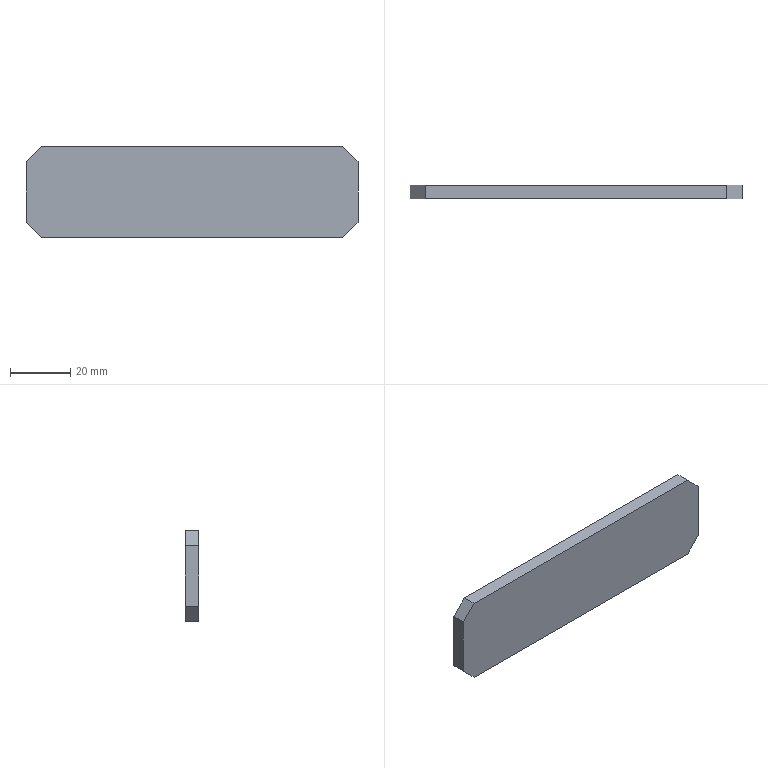Part | SolidWorks | features FlatPattern 1, SMBaseFlange 1, SheetMetal 1 | 1 solid | 10 faces | box 110 x 4.5 x 30 mm | volume 14625 mm3 | plane 10
STEP:
#1=CARTESIAN_POINT('',(-55.,0.,-10.));
#2=VERTEX_POINT('',#1);
#3=CARTESIAN_POINT('',(-55.,0.,10.));
#4=VERTEX_POINT('',#3);
#5=CARTESIAN_POINT('',(-55.,0.,-10.));
#6=DIRECTION('',(0.,0.,1.));
#7=VECTOR('',#6,1000.);
#8=LINE('',#5,#7);
#9=EDGE_CURVE('',#2,#4,#8,.T.);
#10=ORIENTED_EDGE('',*,*,#9,.F.);
#11=CARTESIAN_POINT('',(-55.,-4.5,-10.));
#12=VERTEX_POINT('',#11);
#13=CARTESIAN_POINT('',(-55.,-4.5,-10.));
#14=DIRECTION('',(0.,1.,0.));
#15=VECTOR('',#14,1000.);
#16=LINE('',#13,#15);
#17=EDGE_CURVE('',#12,#2,#16,.T.);
#18=ORIENTED_EDGE('',*,*,#17,.F.);
#19=CARTESIAN_POINT('',(-55.,-4.5,10.));
#20=VERTEX_POINT('',#19);
#21=CARTESIAN_POINT('',(-55.,-4.5,-10.));
#22=DIRECTION('',(0.,0.,1.));
#23=VECTOR('',#22,1000.);
#24=LINE('',#21,#23);
#25=EDGE_CURVE('',#12,#20,#24,.T.);
#26=ORIENTED_EDGE('',*,*,#25,.T.);
#27=CARTESIAN_POINT('',(-55.,-4.5,10.));
#28=DIRECTION('',(0.,1.,0.));
#29=VECTOR('',#28,1000.);
#30=LINE('',#27,#29);
#31=EDGE_CURVE('',#20,#4,#30,.T.);
#32=ORIENTED_EDGE('',*,*,#31,.T.);
#33=EDGE_LOOP('',(#10,#18,#26,#32));
#34=FACE_OUTER_BOUND('',#33,.T.);
#35=CARTESIAN_POINT('',(-55.,-4.5,-10.));
#36=DIRECTION('',(-1.,0.,0.));
#37=DIRECTION('',(0.,0.,1.));
#38=AXIS2_PLACEMENT_3D('',#35,#36,#37);
#39=PLANE('',#38);
#40=ADVANCED_FACE('',(#34),#39,.T.);
#41=CARTESIAN_POINT('',(-50.,0.,-15.));
#42=VERTEX_POINT('',#41);
#43=CARTESIAN_POINT('',(-55.,0.,-10.));
#44=DIRECTION('',(-0.7071,0.,0.7071));
#45=VECTOR('',#44,1000.);
#46=LINE('',#43,#45);
#47=EDGE_CURVE('',#42,#2,#46,.T.);
#48=ORIENTED_EDGE('',*,*,#47,.F.);
#49=CARTESIAN_POINT('',(-50.,-4.5,-15.));
#50=VERTEX_POINT('',#49);
#51=CARTESIAN_POINT('',(-50.,-4.5,-15.));
#52=DIRECTION('',(0.,1.,0.));
#53=VECTOR('',#52,1000.);
#54=LINE('',#51,#53);
#55=EDGE_CURVE('',#50,#42,#54,.T.);
#56=ORIENTED_EDGE('',*,*,#55,.F.);
#57=CARTESIAN_POINT('',(-55.,-4.5,-10.));
#58=DIRECTION('',(-0.7071,0.,0.7071));
#59=VECTOR('',#58,1000.);
#60=LINE('',#57,#59);
#61=EDGE_CURVE('',#50,#12,#60,.T.);
#62=ORIENTED_EDGE('',*,*,#61,.T.);
#63=ORIENTED_EDGE('',*,*,#17,.T.);
#64=EDGE_LOOP('',(#48,#56,#62,#63));
#65=FACE_OUTER_BOUND('',#64,.T.);
#66=CARTESIAN_POINT('',(-55.,-4.5,-10.));
#67=DIRECTION('',(-0.7071,0.,-0.7071));
#68=DIRECTION('',(-0.7071,0.,0.7071));
#69=AXIS2_PLACEMENT_3D('',#66,#67,#68);
#70=PLANE('',#69);
#71=ADVANCED_FACE('',(#65),#70,.T.);
#72=CARTESIAN_POINT('',(50.,0.,-15.));
#73=VERTEX_POINT('',#72);
#74=CARTESIAN_POINT('',(-50.,0.,-15.));
#75=DIRECTION('',(-1.,0.,0.));
#76=VECTOR('',#75,1000.);
#77=LINE('',#74,#76);
#78=EDGE_CURVE('',#73,#42,#77,.T.);
#79=ORIENTED_EDGE('',*,*,#78,.F.);
#80=CARTESIAN_POINT('',(50.,-4.5,-15.));
#81=VERTEX_POINT('',#80);
#82=CARTESIAN_POINT('',(50.,-4.5,-15.));
#83=DIRECTION('',(0.,1.,0.));
#84=VECTOR('',#83,1000.);
#85=LINE('',#82,#84);
#86=EDGE_CURVE('',#81,#73,#85,.T.);
#87=ORIENTED_EDGE('',*,*,#86,.F.);
#88=CARTESIAN_POINT('',(-50.,-4.5,-15.));
#89=DIRECTION('',(-1.,0.,0.));
#90=VECTOR('',#89,1000.);
#91=LINE('',#88,#90);
#92=EDGE_CURVE('',#81,#50,#91,.T.);
#93=ORIENTED_EDGE('',*,*,#92,.T.);
#94=ORIENTED_EDGE('',*,*,#55,.T.);
#95=EDGE_LOOP('',(#79,#87,#93,#94));
#96=FACE_OUTER_BOUND('',#95,.T.);
#97=CARTESIAN_POINT('',(-50.,-4.5,-15.));
#98=DIRECTION('',(0.,0.,-1.));
#99=DIRECTION('',(-1.,0.,0.));
#100=AXIS2_PLACEMENT_3D('',#97,#98,#99);
#101=PLANE('',#100);
#102=ADVANCED_FACE('',(#96),#101,.T.);
#103=CARTESIAN_POINT('',(55.,0.,-10.));
#104=VERTEX_POINT('',#103);
#105=CARTESIAN_POINT('',(50.,0.,-15.));
#106=DIRECTION('',(-0.7071,0.,-0.7071));
#107=VECTOR('',#106,1000.);
#108=LINE('',#105,#107);
#109=EDGE_CURVE('',#104,#73,#108,.T.);
#110=ORIENTED_EDGE('',*,*,#109,.F.);
#111=CARTESIAN_POINT('',(55.,-4.5,-10.));
#112=VERTEX_POINT('',#111);
#113=CARTESIAN_POINT('',(55.,-4.5,-10.));
#114=DIRECTION('',(0.,1.,0.));
#115=VECTOR('',#114,1000.);
#116=LINE('',#113,#115);
#117=EDGE_CURVE('',#112,#104,#116,.T.);
#118=ORIENTED_EDGE('',*,*,#117,.F.);
#119=CARTESIAN_POINT('',(50.,-4.5,-15.));
#120=DIRECTION('',(-0.7071,0.,-0.7071));
#121=VECTOR('',#120,1000.);
#122=LINE('',#119,#121);
#123=EDGE_CURVE('',#112,#81,#122,.T.);
#124=ORIENTED_EDGE('',*,*,#123,.T.);
#125=ORIENTED_EDGE('',*,*,#86,.T.);
#126=EDGE_LOOP('',(#110,#118,#124,#125));
#127=FACE_OUTER_BOUND('',#126,.T.);
#128=CARTESIAN_POINT('',(50.,-4.5,-15.));
#129=DIRECTION('',(0.7071,0.,-0.7071));
#130=DIRECTION('',(-0.7071,0.,-0.7071));
#131=AXIS2_PLACEMENT_3D('',#128,#129,#130);
#132=PLANE('',#131);
#133=ADVANCED_FACE('',(#127),#132,.T.);
#134=CARTESIAN_POINT('',(55.,0.,10.));
#135=VERTEX_POINT('',#134);
#136=CARTESIAN_POINT('',(55.,0.,-10.));
#137=DIRECTION('',(0.,0.,-1.));
#138=VECTOR('',#137,1000.);
#139=LINE('',#136,#138);
#140=EDGE_CURVE('',#135,#104,#139,.T.);
#141=ORIENTED_EDGE('',*,*,#140,.F.);
#142=CARTESIAN_POINT('',(55.,-4.5,10.));
#143=VERTEX_POINT('',#142);
#144=CARTESIAN_POINT('',(55.,-4.5,10.));
#145=DIRECTION('',(0.,1.,0.));
#146=VECTOR('',#145,1000.);
#147=LINE('',#144,#146);
#148=EDGE_CURVE('',#143,#135,#147,.T.);
#149=ORIENTED_EDGE('',*,*,#148,.F.);
#150=CARTESIAN_POINT('',(55.,-4.5,-10.));
#151=DIRECTION('',(0.,0.,-1.));
#152=VECTOR('',#151,1000.);
#153=LINE('',#150,#152);
#154=EDGE_CURVE('',#143,#112,#153,.T.);
#155=ORIENTED_EDGE('',*,*,#154,.T.);
#156=ORIENTED_EDGE('',*,*,#117,.T.);
#157=EDGE_LOOP('',(#141,#149,#155,#156));
#158=FACE_OUTER_BOUND('',#157,.T.);
#159=CARTESIAN_POINT('',(55.,-4.5,-10.));
#160=DIRECTION('',(1.,0.,0.));
#161=DIRECTION('',(0.,0.,-1.));
#162=AXIS2_PLACEMENT_3D('',#159,#160,#161);
#163=PLANE('',#162);
#164=ADVANCED_FACE('',(#158),#163,.T.);
#165=CARTESIAN_POINT('',(50.,0.,15.));
#166=VERTEX_POINT('',#165);
#167=CARTESIAN_POINT('',(50.,0.,15.));
#168=DIRECTION('',(0.7071,0.,-0.7071));
#169=VECTOR('',#168,1000.);
#170=LINE('',#167,#169);
#171=EDGE_CURVE('',#166,#135,#170,.T.);
#172=ORIENTED_EDGE('',*,*,#171,.F.);
#173=CARTESIAN_POINT('',(50.,-4.5,15.));
#174=VERTEX_POINT('',#173);
#175=CARTESIAN_POINT('',(50.,-4.5,15.));
#176=DIRECTION('',(0.,1.,0.));
#177=VECTOR('',#176,1000.);
#178=LINE('',#175,#177);
#179=EDGE_CURVE('',#174,#166,#178,.T.);
#180=ORIENTED_EDGE('',*,*,#179,.F.);
#181=CARTESIAN_POINT('',(50.,-4.5,15.));
#182=DIRECTION('',(0.7071,0.,-0.7071));
#183=VECTOR('',#182,1000.);
#184=LINE('',#181,#183);
#185=EDGE_CURVE('',#174,#143,#184,.T.);
#186=ORIENTED_EDGE('',*,*,#185,.T.);
#187=ORIENTED_EDGE('',*,*,#148,.T.);
#188=EDGE_LOOP('',(#172,#180,#186,#187));
#189=FACE_OUTER_BOUND('',#188,.T.);
#190=CARTESIAN_POINT('',(50.,-4.5,15.));
#191=DIRECTION('',(0.7071,0.,0.7071));
#192=DIRECTION('',(0.7071,0.,-0.7071));
#193=AXIS2_PLACEMENT_3D('',#190,#191,#192);
#194=PLANE('',#193);
#195=ADVANCED_FACE('',(#189),#194,.T.);
#196=CARTESIAN_POINT('',(-50.,0.,15.));
#197=VERTEX_POINT('',#196);
#198=CARTESIAN_POINT('',(-50.,0.,15.));
#199=DIRECTION('',(1.,0.,0.));
#200=VECTOR('',#199,1000.);
#201=LINE('',#198,#200);
#202=EDGE_CURVE('',#197,#166,#201,.T.);
#203=ORIENTED_EDGE('',*,*,#202,.F.);
#204=CARTESIAN_POINT('',(-50.,-4.5,15.));
#205=VERTEX_POINT('',#204);
#206=CARTESIAN_POINT('',(-50.,-4.5,15.));
#207=DIRECTION('',(0.,1.,0.));
#208=VECTOR('',#207,1000.);
#209=LINE('',#206,#208);
#210=EDGE_CURVE('',#205,#197,#209,.T.);
#211=ORIENTED_EDGE('',*,*,#210,.F.);
#212=CARTESIAN_POINT('',(-50.,-4.5,15.));
#213=DIRECTION('',(1.,0.,0.));
#214=VECTOR('',#213,1000.);
#215=LINE('',#212,#214);
#216=EDGE_CURVE('',#205,#174,#215,.T.);
#217=ORIENTED_EDGE('',*,*,#216,.T.);
#218=ORIENTED_EDGE('',*,*,#179,.T.);
#219=EDGE_LOOP('',(#203,#211,#217,#218));
#220=FACE_OUTER_BOUND('',#219,.T.);
#221=CARTESIAN_POINT('',(-50.,-4.5,15.));
#222=DIRECTION('',(0.,0.,1.));
#223=DIRECTION('',(1.,0.,0.));
#224=AXIS2_PLACEMENT_3D('',#221,#222,#223);
#225=PLANE('',#224);
#226=ADVANCED_FACE('',(#220),#225,.T.);
#227=CARTESIAN_POINT('',(-55.,0.,10.));
#228=DIRECTION('',(0.7071,0.,0.7071));
#229=VECTOR('',#228,1000.);
#230=LINE('',#227,#229);
#231=EDGE_CURVE('',#4,#197,#230,.T.);
#232=ORIENTED_EDGE('',*,*,#231,.F.);
#233=ORIENTED_EDGE('',*,*,#31,.F.);
#234=CARTESIAN_POINT('',(-55.,-4.5,10.));
#235=DIRECTION('',(0.7071,0.,0.7071));
#236=VECTOR('',#235,1000.);
#237=LINE('',#234,#236);
#238=EDGE_CURVE('',#20,#205,#237,.T.);
#239=ORIENTED_EDGE('',*,*,#238,.T.);
#240=ORIENTED_EDGE('',*,*,#210,.T.);
#241=EDGE_LOOP('',(#232,#233,#239,#240));
#242=FACE_OUTER_BOUND('',#241,.T.);
#243=CARTESIAN_POINT('',(-55.,-4.5,10.));
#244=DIRECTION('',(-0.7071,0.,0.7071));
#245=DIRECTION('',(0.7071,0.,0.7071));
#246=AXIS2_PLACEMENT_3D('',#243,#244,#245);
#247=PLANE('',#246);
#248=ADVANCED_FACE('',(#242),#247,.T.);
#249=ORIENTED_EDGE('',*,*,#25,.F.);
#250=ORIENTED_EDGE('',*,*,#61,.F.);
#251=ORIENTED_EDGE('',*,*,#92,.F.);
#252=ORIENTED_EDGE('',*,*,#123,.F.);
#253=ORIENTED_EDGE('',*,*,#154,.F.);
#254=ORIENTED_EDGE('',*,*,#185,.F.);
#255=ORIENTED_EDGE('',*,*,#216,.F.);
#256=ORIENTED_EDGE('',*,*,#238,.F.);
#257=EDGE_LOOP('',(#249,#250,#251,#252,#253,#254,#255,#256));
#258=FACE_OUTER_BOUND('',#257,.T.);
#259=CARTESIAN_POINT('',(0.,-4.5,0.));
#260=DIRECTION('',(0.,1.,0.));
#261=DIRECTION('',(0.,0.,1.));
#262=AXIS2_PLACEMENT_3D('',#259,#260,#261);
#263=PLANE('',#262);
#264=ADVANCED_FACE('',(#258),#263,.F.);
#265=ORIENTED_EDGE('',*,*,#9,.T.);
#266=ORIENTED_EDGE('',*,*,#231,.T.);
#267=ORIENTED_EDGE('',*,*,#202,.T.);
#268=ORIENTED_EDGE('',*,*,#171,.T.);
#269=ORIENTED_EDGE('',*,*,#140,.T.);
#270=ORIENTED_EDGE('',*,*,#109,.T.);
#271=ORIENTED_EDGE('',*,*,#78,.T.);
#272=ORIENTED_EDGE('',*,*,#47,.T.);
#273=EDGE_LOOP('',(#265,#266,#267,#268,#269,#270,#271,#272));
#274=FACE_OUTER_BOUND('',#273,.T.);
#275=CARTESIAN_POINT('',(0.,0.,0.));
#276=DIRECTION('',(0.,1.,0.));
#277=DIRECTION('',(0.,0.,1.));
#278=AXIS2_PLACEMENT_3D('',#275,#276,#277);
#279=PLANE('',#278);
#280=ADVANCED_FACE('',(#274),#279,.T.);
#281=CLOSED_SHELL('',(#40,#71,#102,#133,#164,#195,#226,#248,#264,#280));
#282=MANIFOLD_SOLID_BREP('',#281);
#283=CARTESIAN_POINT('',(0.,0.,0.));
#284=DIRECTION('',(0.,0.,1.));
#285=DIRECTION('',(1.,0.,0.));
#286=AXIS2_PLACEMENT_3D('',#283,#284,#285);
#287=(LENGTH_UNIT()NAMED_UNIT(*)SI_UNIT(.MILLI.,.METRE.));
#288=UNCERTAINTY_MEASURE_WITH_UNIT(LENGTH_MEASURE(0.00001),#287,'','');
#289=(NAMED_UNIT(*)PLANE_ANGLE_UNIT()SI_UNIT($,.RADIAN.));
#290=(NAMED_UNIT(*)SI_UNIT($,.STERADIAN.)SOLID_ANGLE_UNIT());
#291=(GEOMETRIC_REPRESENTATION_CONTEXT(3)GLOBAL_UNCERTAINTY_ASSIGNED_CONTEXT((#288))GLOBAL_UNIT_ASSIGNED_CONTEXT((#287,#289,#290))REPRESENTATION_CONTEXT('',''));
#292=ADVANCED_BREP_SHAPE_REPRESENTATION('',(#282,#286),#291);